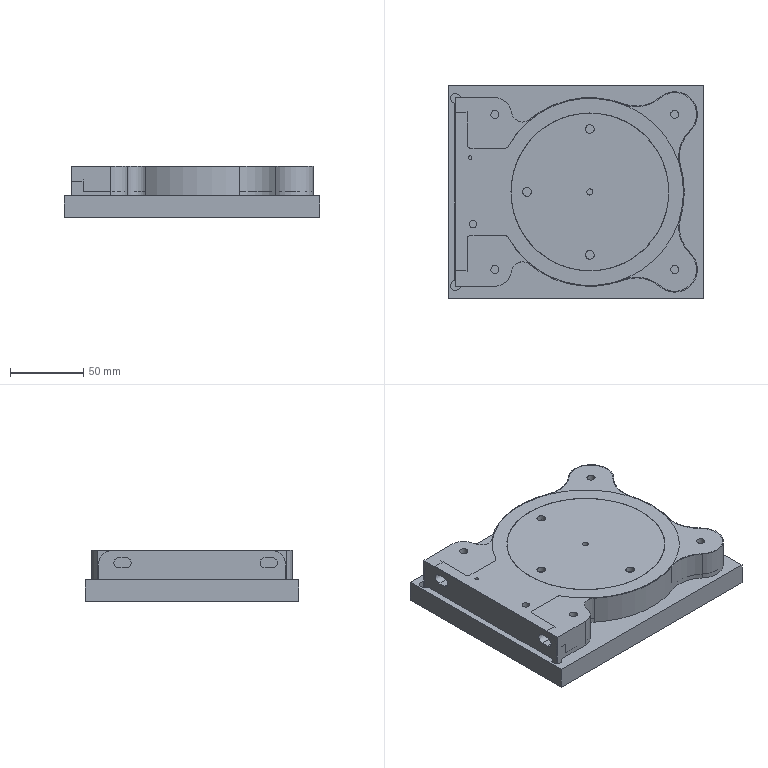NC program | NX | posted with a generic post | part box 175 x 146 x 35 mm
Lines 2956 to 4708 of 35144, first 1512 of 1711 lines:
(打点_COPY_COPY , TOOL : DJ6)
N5898 T12 M6
N5900 G54
N5902 G17 G0 G90 X67.5 Y-53. S3000 M3
N5904 G43 Z20. H12
N5906 G94 G81 G98 Z-1.2 F200. R3.
N5908 X-55.5
N5910 Y53.
N5912 X67.5
N5914 X9.5 Y0.
N5916 G80
N5918 G0 X9.5 Y0. Z20.
N5920 M5
(DRILLING_COPY_1 , TOOL : Z4.3)
N5922 T16 M6
N5924 G54
N5926 G17 G0 G90 X67.5 Y53. S3000 M3
N5928 G43 Z20. H16
N5930 G94 G83 G98 Z-15. F200. Q3. R3.
N5932 Y-53.
N5934 X9.5 Y0.
N5936 X-55.5 Y-53.
N5938 Y53.
N5940 G80
N5942 G0 X-55.5 Y53. Z20.
N5944 M5
(打点_COPY_COPY_COPY , TOOL : DJ6)
N5946 T12 M6
N5948 G54
N5950 G17 G0 G90 X67.5 Y-53. S3000 M3
N5952 G43 Z20. H12
N5954 G94 G81 G98 Z-2.5 F200. R3.
N5956 X-55.5
N5958 Y53.
N5960 X67.5
N5962 X9.5 Y0.
N5964 G80
N5966 G0 X9.5 Y0. Z20.
(倒角_COPY_1_COPY_2 , TOOL : DJ6)
N5968 X-73.2 Y0.249 S7500
N5970 Z-0.5
N5972 G1 Z-1. F1500.
N5974 G3 X-73.7 Y-0.251 R0.5
N5976 G1 Y-24.503
N5978 G2 X-73.993 Y-25.21 R1.
N5980 G1 X-74.288 Y-25.505
N5982 G3 X-74.288 Y-25.788 R0.2
N5984 X-74.005 Y-25.788 R0.2
N5986 G1 X-73.71 Y-25.493
N5988 G2 X-73.003 Y-25.2 R1.
N5990 G1 X-44.7
N5992 G2 X-43.799 Y-25.765 R1.
N5994 G3 X-43.799 Y25.765 R-59.2
N5996 G2 X-44.7 Y25.2 R1.
N5998 G1 X-72.5
N6000 G3 X-73.7 Y24. R1.2
N6002 G1 Y-0.251
N6004 G3 X-73.2 Y-0.751 R0.5
N6006 G1 Z-0.5
N6008 G0 Z20.
(倒角_COPY_1_COPY_2_COPY , TOOL : DJ6)
N6010 X-83.8 Y-0.5
N6012 Z-0.5
N6014 G1 Z-1.
N6016 G3 X-83.3 Y0. R0.5
N6018 G1 Y63.8
N6020 G2 X-82.3 Y64.8 R1.
N6022 G1 X-55.5
N6024 G2 X-43.785 Y54.413 R11.8
N6026 G3 X-32.023 Y49.748 R7.2
N6028 G2 X32.595 Y60.545 R64.8
N6030 G3 X57.119 Y64.911 R24.2
N6032 G2 X78.43 Y41.59 R15.8
N6034 G3 X71.876 Y17.558 R24.2
N6036 G2 X71.876 Y-17.558 R64.8
N6038 G3 X78.43 Y-41.59 R24.2
N6040 G2 X57.119 Y-64.911 R15.8
N6042 G3 X32.595 Y-60.545 R24.2
N6044 G2 X-32.023 Y-49.748 R64.8
N6046 G3 X-43.785 Y-54.413 R7.2
N6048 G2 X-55.5 Y-64.8 R11.8
N6050 G1 X-82.3
N6052 G2 X-83.3 Y-63.8 R1.
N6054 G1 Y0.
N6056 G3 X-83.8 Y0.5 R0.5
N6058 G1 Z-0.5
N6060 G0 Z20.
N6062 M5
(DRILLING_COPY_1_COPY , TOOL : M5)
N6064 T20 M6
N6066 G54
N6068 G17 G0 G90 X67.5 Y53. S300 M3
N6070 G43 Z20. H20
N6072 G84 G94 G98 Z-13. F72000. R3.
N6074 Y-53.
N6076 X9.5 Y0.
N6078 X-55.5 Y-53.
N6080 Y53.
N6082 G80
N6084 G0 X-55.5 Y53. Z20.
N6086 M5
(正面_COPY_COPY , TOOL : D10)
N6088 T02 M6
N6090 G54
N6092 G17 G0 G90 X95.5 Y-68.762 S8000 M3
N6094 G43 Z20. H2
N6096 Z0.1
N6098 G94 G1 X90.5 F1500.
N6100 X-90.5
N6102 Y-61.524
N6104 X90.5
N6106 Y-54.286
N6108 X-90.5
N6110 Y-47.048
N6112 X90.5
N6114 Y-39.81
N6116 X-90.5
N6118 Y-32.571
N6120 X90.5
N6122 Y-25.333
N6124 X-90.5
N6126 Y-18.095
N6128 X90.5
N6130 Y-10.857
N6132 X-90.5
N6134 Y-3.619
N6136 X90.5
N6138 Y3.619
N6140 X-90.5
N6142 Y10.857
N6144 X90.5
N6146 Y18.095
N6148 X-90.5
N6150 Y25.333
N6152 X90.5
N6154 Y32.571
N6156 X-90.5
N6158 Y39.81
N6160 X90.5
N6162 Y47.048
N6164 X-90.5
N6166 Y54.286
N6168 X90.5
N6170 Y61.524
N6172 X-90.5
N6174 Y68.762
N6176 X90.5
N6178 X95.5
N6180 G0 Z20.
(跟随部件_COPY_1_COPY_1 , TOOL : D10)
N6182 G1 X84.885 Y-72.393 F15000.
N6184 Z-26.5
N6186 Z-27. F1500.
N6188 G3 X78.03 Y-70.659 R5.
N6190 G2 X53.992 Y-68.5 R20.56
N6192 G3 X34.291 Y-64.992 R19.44
N6194 G2 X-35.073 Y-53.402 R69.56
N6196 G3 X-39.059 Y-54.983 R2.44
N6198 G2 X-55.5 Y-69.56 R16.56
N6200 G1 X-82.5
N6202 G2 X-88.06 Y-64. R5.56
N6204 G1 Y64.
N6206 G2 X-82.5 Y69.56 R5.56
N6208 G1 X-55.5
N6210 G2 X-39.059 Y54.983 R16.56
N6212 G3 X-35.073 Y53.402 R2.44
N6214 G2 X34.291 Y64.992 R69.56
N6216 G3 X53.992 Y68.5 R19.44
N6218 G2 X81.723 Y38.153 R20.56
N6220 G3 X76.458 Y18.848 R19.44
N6222 G2 X76.458 Y-18.848 R69.56
N6224 G3 X81.723 Y-38.153 R19.44
N6226 G2 X77.597 Y-70.91 R20.56
N6228 G3 X75.697 Y-77.721 R5.
N6230 G1 X84.854 Y-72.341
N6232 G3 X77.999 Y-70.607 R5.
N6234 G2 X54.031 Y-68.455 R20.5
N6236 G3 X34.27 Y-64.936 R19.5
N6238 G2 X-35.035 Y-53.356 R69.5
N6240 G3 X-39.119 Y-54.976 R2.5
N6242 G2 X-55.5 Y-69.5 R16.5
N6244 G1 X-82.5
N6246 G2 X-88. Y-64. R5.5
N6248 G1 Y64.
N6250 G2 X-82.5 Y69.5 R5.5
N6252 G1 X-55.5
N6254 G2 X-39.119 Y54.976 R16.5
N6256 G3 X-35.035 Y53.356 R2.5
N6258 G2 X34.27 Y64.936 R69.5
N6260 G3 X54.031 Y68.455 R19.5
N6262 G2 X81.681 Y38.197 R20.5
N6264 G3 X76.4 Y18.831 R19.5
N6266 G2 X76.4 Y-18.831 R69.5
N6268 G3 X81.681 Y-38.197 R19.5
N6270 G2 X77.999 Y-70.607 R20.5
N6272 X77.566 Y-70.858 R20.5
N6274 G3 X75.666 Y-77.669 R5.
N6276 G1 Z-26.5
N6278 Z20. F15000.
(反面_COPY , TOOL : D10)
N6280 G0 X-71.818 Y-98.5
N6282 Z3.4
N6284 G1 Y-93.5 F4000.
N6286 Y93.5
N6288 X-64.636
N6290 Y-93.5
N6292 X-57.455
N6294 Y93.5
N6296 X-50.273
N6298 Y-93.5
N6300 X-43.091
N6302 Y93.5
N6304 X-35.909
N6306 Y-93.5
N6308 X-28.727
N6310 Y93.5
N6312 X-21.545
N6314 Y-93.5
N6316 X-14.364
N6318 Y93.5
N6320 X-7.182
N6322 Y-93.5
N6324 X0.
N6326 Y93.5
N6328 X7.182
N6330 Y-93.5
N6332 X14.364
N6334 Y93.5
N6336 X21.545
N6338 Y-93.5
N6340 X28.727
N6342 Y93.5
N6344 X35.909
N6346 Y-93.5
N6348 X43.091
N6350 Y93.5
N6352 X50.273
N6354 Y-93.5
N6356 X57.455
N6358 Y93.5
N6360 X64.636
N6362 Y-93.5
N6364 X71.818
N6366 Y93.5
N6368 Y98.5
N6370 G0 Z8.
N6372 X-71.818 Y-98.5
N6374 Z1.8
N6376 G1 Y-93.5
N6378 Y93.5
N6380 X-64.636
N6382 Y-93.5
N6384 X-57.455
N6386 Y93.5
N6388 X-50.273
N6390 Y-93.5
N6392 X-43.091
N6394 Y93.5
N6396 X-35.909
N6398 Y-93.5
N6400 X-28.727
N6402 Y93.5
N6404 X-21.545
N6406 Y-93.5
N6408 X-14.364
N6410 Y93.5
N6412 X-7.182
N6414 Y-93.5
N6416 X0.
N6418 Y93.5
N6420 X7.182
N6422 Y-93.5
N6424 X14.364
N6426 Y93.5
N6428 X21.545
N6430 Y-93.5
N6432 X28.727
N6434 Y93.5
N6436 X35.909
N6438 Y-93.5
N6440 X43.091
N6442 Y93.5
N6444 X50.273
N6446 Y-93.5
N6448 X57.455
N6450 Y93.5
N6452 X64.636
N6454 Y-93.5
N6456 X71.818
N6458 Y93.5
N6460 Y98.5
N6462 G0 Z6.4
N6464 X-71.818 Y-98.5
N6466 Z0.2
N6468 G1 Y-93.5
N6470 Y93.5
N6472 X-64.636
N6474 Y-93.5
N6476 X-57.455
N6478 Y93.5
N6480 X-50.273
N6482 Y-93.5
N6484 X-43.091
N6486 Y93.5
N6488 X-35.909
N6490 Y-93.5
N6492 X-28.727
N6494 Y93.5
N6496 X-21.545
N6498 Y-93.5
N6500 X-14.364
N6502 Y93.5
N6504 X-7.182
N6506 Y-93.5
N6508 X0.
N6510 Y93.5
N6512 X7.182
N6514 Y-93.5
N6516 X14.364
N6518 Y93.5
N6520 X21.545
N6522 Y-93.5
N6524 X28.727
N6526 Y93.5
N6528 X35.909
N6530 Y-93.5
N6532 X43.091
N6534 Y93.5
N6536 X50.273
N6538 Y-93.5
N6540 X57.455
N6542 Y93.5
N6544 X64.636
N6546 Y-93.5
N6548 X71.818
N6550 Y93.5
N6552 Y98.5
N6554 G0 Z20.
(反面_COPY_COPY , TOOL : D10)
N6556 X-70.571 Y-97.5
N6558 Z0.1
N6560 G1 Y-92.5 F2000.
N6562 Y92.5
N6564 X-63.143
N6566 Y-92.5
N6568 X-55.714
N6570 Y92.5
N6572 X-48.286
N6574 Y-92.5
N6576 X-40.857
N6578 Y92.5
N6580 X-33.429
N6582 Y-92.5
N6584 X-26.
N6586 Y92.5
N6588 X-18.571
N6590 Y-92.5
N6592 X-11.143
N6594 Y92.5
N6596 X-3.714
N6598 Y-92.5
N6600 X3.714
N6602 Y92.5
N6604 X11.143
N6606 Y-92.5
N6608 X18.571
N6610 Y92.5
N6612 X26.
N6614 Y-92.5
N6616 X33.429
N6618 Y92.5
N6620 X40.857
N6622 Y-92.5
N6624 X48.286
N6626 Y92.5
N6628 X55.714
N6630 Y-92.5
N6632 X63.143
N6634 Y92.5
N6636 X70.571
N6638 Y-92.5
N6640 Y-97.5
N6642 G0 Z20.
N6644 M5
(打点_COPY_COPY_COPY_1 , TOOL : DJ8)
N6646 T12 M6
N6648 G54
N6650 G17 G0 G90 X53. Y-67.5 S3000 M3
N6652 G43 Z20. H12
N6654 G94 G81 G98 Z-1.2 F200. R3.
N6656 X-53.
N6658 X0. Y-9.5
N6660 X-53. Y55.5
N6662 X-22. Y70.5
N6664 X53. Y55.5
N6666 G80
N6668 G0 X53. Y55.5 Z20.
N6670 M5
(DRILLING_COPY_1_COPY_1 , TOOL : Z4.3)
N6672 T16 M6
N6674 G54
N6676 G17 G0 G90 X0. Y-9.5 S3000 M3
N6678 G43 Z20. H16
N6680 G94 G83 G98 Z-15. F200. Q3. R3.
N6682 G80
N6684 G0 X0. Y-9.5 Z20.
(DRILLING_COPY_1_COPY_1_COPY_1 , TOOL : Z4.3)
N6686 X53. Y-67.5
N6688 G83 Z-15. F200. Q3. R3.
N6690 X-53.
N6692 X53. Y55.5
N6694 X-53.
N6696 G80
N6698 G0 X-53. Y55.5 Z20.
N6700 M5
(打点_COPY_COPY_COPY_COPY , TOOL : DJ8)
N6702 T12 M6
N6704 G54
N6706 G17 G0 G90 X0. Y-9.5 S3000 M3
N6708 G43 Z20. H12
N6710 G94 G81 G98 Z-2.5 F200. R3.
N6712 X53. Y-67.5
N6714 X-53.
N6716 G80
N6718 G0 X-53. Y-67.5 Z20.
(打点_COPY_COPY_COPY_COPY_COPY , TOOL : DJ8)
N6720 X53. Y55.5
N6722 G81 Z-2.5 F200. R3.
N6724 X-53.
N6726 X-22. Y70.5
N6728 G80
N6730 G0 X-22. Y70.5 Z20.
(倒角_COPY_1_COPY_2_COPY_1 , TOOL : DJ8)
N6732 X-1. Y84.3 S7500
N6734 Z-0.5
N6736 G1 Z-1. F1500.
N6738 G3 X0. Y83.3 R1.
N6740 G1 X64.3
N6742 G2 X65.3 Y82.3 R1.
N6744 G1 Y55.5
N6746 G2 X54.473 Y43.289 R12.3
N6748 G3 X50.132 Y32.343 R6.7
N6750 G2 X61.012 Y-32.773 R65.3
N6752 G3 X65.288 Y-56.791 R23.7
N6754 G2 X41.229 Y-78.776 R16.3
N6756 G3 X17.693 Y-72.357 R23.7
N6758 G2 X-17.693 Y-72.357 R65.3
N6760 G3 X-41.229 Y-78.776 R23.7
N6762 G2 X-65.288 Y-56.791 R16.3
N6764 G3 X-61.012 Y-32.773 R23.7
N6766 G2 X-50.132 Y32.343 R65.3
N6768 G3 X-54.473 Y43.289 R6.7
N6770 G2 X-65.3 Y55.5 R12.3
N6772 G1 Y82.3
N6774 G2 X-64.3 Y83.3 R1.
N6776 G1 X0.
N6778 G3 X1. Y84.3 R1.
N6780 G1 Z-0.5
N6782 G0 Z20.
N6784 M5
(DRILLING_COPY_1_COPY_COPY , TOOL : M5)
N6786 T20 M6
N6788 G54
N6790 G17 G0 G90 X-53. Y-67.5 S300 M3
N6792 G43 Z20. H20
N6794 G84 G94 G98 Z-13.5 F72000. R3.
N6796 X53.
N6798 X0. Y-9.5
N6800 X53. Y55.5
N6802 X-53.
N6804 G80
N6806 G0 X-53. Y55.5 Z20.
N6808 M5
(跟随部件_COPY_3 , TOOL : D10)
N6810 T02 M6
N6812 G54
N6814 G17 G94 G1 G90 X-1.729 Y-10.159 F15000. S8000 M3
N6816 G43 Z20. H2
N6818 Z0.22
N6820 X-1.562 Y-10.595 Z0.204 F4000.
N6822 X-1.401 Y-11.033 Z0.187
N6824 X-0.95 Y-11.154 Z0.171
N6826 X-0.501 Y-11.281 Z0.155
N6828 X-0.179 Y-11.371 Z0.143
N6830 X0.179 Y-11.372 Z0.131
N6832 X0.501 Y-11.281 Z0.119
N6834 X0.95 Y-11.154 Z0.103
N6836 X1.401 Y-11.033 Z0.086
N6838 X1.562 Y-10.595 Z0.07
N6840 X1.729 Y-10.159 Z0.054
N6842 X1.848 Y-9.847 Z0.042
N6844 X1.854 Y-9.19 Z0.019
N6846 X1.635 Y-8.571 Z-0.004
N6848 X1.058 Y-7.881 Z-0.035
N6850 X0.348 Y-7.001 Z-0.075
N6852 X0. Y-6.556 Z-0.094
N6854 X-0.696 Y-7.447 Z-0.134
N6856 X-1.42 Y-8.315 Z-0.173
N6858 X-1.635 Y-8.571 Z-0.185
N6860 X-1.854 Y-9.19 Z-0.208
N6862 X-1.848 Y-9.847 Z-0.231
N6864 X-1.729 Y-10.159 Z-0.243
N6866 X-1.562 Y-10.595 Z-0.259
N6868 X-1.401 Y-11.033 Z-0.275
N6870 X-0.95 Y-11.154 Z-0.291
N6872 X-0.501 Y-11.281 Z-0.308
N6874 X-0.179 Y-11.371 Z-0.319
N6876 X0.179 Y-11.372 Z-0.332
N6878 X0.501 Y-11.281 Z-0.344
N6880 X0.95 Y-11.154 Z-0.36
N6882 X1.401 Y-11.033 Z-0.376
N6884 X1.562 Y-10.595 Z-0.392
N6886 X1.729 Y-10.159 Z-0.409
N6888 X1.848 Y-9.847 Z-0.42
N6890 X1.854 Y-9.19 Z-0.443
N6892 X1.635 Y-8.571 Z-0.466
N6894 X1.058 Y-7.881 Z-0.498
N6896 X0.348 Y-7.001 Z-0.537
N6898 X0. Y-6.556 Z-0.557
N6900 X-0.696 Y-7.447 Z-0.596
N6902 X-1.42 Y-8.315 Z-0.636
N6904 X-1.635 Y-8.571 Z-0.648
N6906 X-1.854 Y-9.19 Z-0.67
N6908 X-1.848 Y-9.847 Z-0.693
N6910 X-1.729 Y-10.159 Z-0.705
N6912 X-1.562 Y-10.595 Z-0.721
N6914 X-1.401 Y-11.033 Z-0.738
N6916 X-0.95 Y-11.154 Z-0.754
N6918 X-0.501 Y-11.281 Z-0.77
N6920 X-0.179 Y-11.371 Z-0.782
N6922 X0.179 Y-11.372 Z-0.794
N6924 X0.501 Y-11.281 Z-0.806
N6926 X0.95 Y-11.154 Z-0.822
N6928 X1.401 Y-11.033 Z-0.839
N6930 X1.562 Y-10.595 Z-0.855
N6932 X1.729 Y-10.159 Z-0.871
N6934 X1.848 Y-9.847 Z-0.883
N6936 X1.854 Y-9.19 Z-0.906
N6938 X1.635 Y-8.571 Z-0.929
N6940 X1.058 Y-7.881 Z-0.96
N6942 X0.703 Y-7.441 Z-0.98
N6944 G2 X0. Y-6.556 R70.15
N6946 X-1.42 Y-8.315 R70.15
N6948 G3 X-1.729 Y-10.159 R1.85
N6950 G2 X-1.401 Y-11.033 R87.15
N6952 X-0.501 Y-11.281 R87.15
N6954 G3 X0.501 Y-11.281 R1.85
N6956 G2 X1.401 Y-11.033 R87.15
N6958 X1.729 Y-10.159 R87.15
N6960 G3 X1.42 Y-8.315 R1.85
N6962 G2 X0.703 Y-7.441 R70.15
N6964 G1 X4.593 Y-4.299
N6966 G2 X0. Y2.153 R65.15
N6968 X-5.259 Y-5.111 R65.15
N6970 G3 X-6.4 Y-11.941 R6.85
N6972 G2 X-5.228 Y-15.221 R82.15
N6974 X-1.856 Y-16.094 R82.15
N6976 G3 X1.855 Y-16.094 R6.85
N6978 G2 X5.228 Y-15.221 R82.15
N6980 X6.4 Y-11.941 R82.15
N6982 G3 X5.259 Y-5.111 R6.85
N6984 G2 X4.593 Y-4.299 R65.15
N6986 G1 X10.427 Y0.413
N6988 G2 X0. Y20.262 R57.65
N6990 G1 X-1.351 Y25.076
N6992 G3 X-0.143 Y35.25 R55.15
N6994 G1 X0.143
N6996 G3 X1.351 Y25.076 R55.15
N6998 X-1.351 Y25.076 R5.
N7000 G1 X0. Y20.262
N7002 G2 X-11.017 Y-0.305 R57.65
N7004 G3 X-13.408 Y-14.614 R14.35
N7006 G2 X-11.113 Y-21.662 R74.65
N7008 X-3.888 Y-23.313 R74.65
N7010 G3 X3.887 Y-23.314 R14.35
N7012 G2 X11.113 Y-21.662 R74.65
N7014 X13.408 Y-14.614 R74.65
N7016 G3 X11.017 Y-0.305 R14.35
N7018 G2 X10.427 Y0.413 R57.65
N7020 G1 X16.262 Y5.126
N7022 G2 X5.256 Y40.25 R50.15
N7024 G1 X-5.256
N7026 G2 X-16.775 Y4.501 R50.15
N7028 G3 X-20.415 Y-17.287 R21.85
N7030 G2 X-17.246 Y-28.373 R67.15
N7032 X-5.92 Y-30.533 R67.15
N7034 G3 X5.919 Y-30.533 R21.85
N7036 G2 X17.246 Y-28.373 R67.15
N7038 X20.415 Y-17.287 R67.15
N7040 G3 X16.775 Y4.501 R21.85
N7042 G2 X16.262 Y5.126 R50.15
N7044 G1 X22.096 Y9.838
N7046 G2 X14.099 Y47.75 R42.65
N7048 G1 X-14.099
N7050 G2 X-22.533 Y9.307 R42.65
N7052 G3 X-27.423 Y-19.96 R29.35
N7054 G2 X-23.778 Y-35.522 R59.65
N7056 X-7.953 Y-37.752 R59.65
N7058 G3 X7.951 Y-37.752 R29.35
N7060 G2 X23.778 Y-35.522 R59.65
N7062 X27.423 Y-19.96 R59.65
N7064 G3 X22.533 Y9.307 R29.35
N7066 G2 X22.096 Y9.838 R42.65
N7068 G1 X27.931 Y14.551
N7070 G2 X25.458 Y55.25 R35.15
N7072 G1 X30.059 Y57.607
N7074 X25.458 Y55.25
N7076 X-25.458
N7078 X-30.059 Y57.607
N7080 X-25.458 Y55.25
N7082 G2 X-28.29 Y14.113 R35.15
N7084 G3 X-34.43 Y-22.633 R36.85
N7086 G2 X-31.055 Y-43.484 R52.15
N7088 X-9.985 Y-44.972 R52.15
N7090 G3 X9.984 Y-44.972 R36.85
N7092 G2 X31.055 Y-43.484 R52.15
N7094 X34.43 Y-22.633 R52.15
N7096 G3 X28.29 Y14.113 R36.85
N7098 G2 X27.931 Y14.551 R35.15
N7100 G1 X33.766 Y19.263
N7102 G2 X44.35 Y62.037 R27.65
N7104 G1 Y62.75
N7106 X-44.35
N7108 Y62.037
N7110 G2 X-34.048 Y18.919 R27.65
N7112 G3 X-41.438 Y-25.306 R44.35
N7114 G2 X-40.237 Y-53.533 R44.65
N7116 G1 X-43.947 Y-57.593
N7118 X-40.237 Y-53.533
N7120 G2 X-12.017 Y-52.191 R44.65
N7122 G3 X12.017 Y-52.191 R44.35
N7124 G2 X40.237 Y-53.533 R44.65
N7126 G1 X43.947 Y-57.593
N7128 X40.237 Y-53.533
N7130 G2 X41.438 Y-25.306 R44.65
N7132 G3 X34.048 Y18.919 R44.35
N7134 G2 X33.766 Y19.263 R27.65
N7136 G1 X39.6 Y23.976
N7138 G2 X51.85 Y56.493 R20.15
N7140 G1 Y70.25
N7142 X-51.85
N7144 Y56.493
N7146 G2 X-39.806 Y23.725 R20.15
N7148 G3 X-48.445 Y-27.98 R51.85
N7150 G2 X-55.149 Y-65.628 R37.15
N7152 G3 X-50.942 Y-69.472 R2.85
N7154 G2 X-14.049 Y-59.41 R37.15
N7156 G3 X14.049 Y-59.41 R51.85
N7158 G2 X50.942 Y-69.472 R37.15
N7160 G3 X55.149 Y-65.628 R2.85
N7162 G2 X48.445 Y-27.98 R37.15
N7164 G3 X39.806 Y23.725 R51.85
N7166 G2 X39.6 Y23.976 R20.15
N7168 G1 X45.435 Y28.688
N7170 G2 X53.761 Y49.196 R12.65
N7172 G3 X59.35 Y55.5 R6.35
N7174 G1 Y77.304
N7176 G2 X59.364 Y77.764 R7.75
N7178 X58.904 Y77.75 R7.75
N7180 G1 X-58.904
N7182 G2 X-59.364 Y77.764 R7.75
N7184 X-59.35 Y77.304 R7.75
N7186 G1 Y55.5
N7188 G3 X-53.761 Y49.196 R6.35
N7190 G2 X-45.564 Y28.531 R12.65
N7192 G3 X-55.453 Y-30.653 R59.35
N7194 G2 X-60.803 Y-60.7 R29.65
N7196 G3 X-45.526 Y-74.66 R10.35
N7198 G2 X-16.081 Y-66.63 R29.65
N7200 G3 X16.081 Y-66.63 R59.35
N7202 G2 X45.526 Y-74.66 R29.65
N7204 G3 X60.803 Y-60.7 R10.35
N7206 G2 X55.453 Y-30.653 R29.65
N7208 G3 X45.564 Y28.531 R59.35
N7210 G2 X45.435 Y28.688 R12.65
N7212 G3 X38.403 Y29.436 R5.
N7214 G1 Z-0.48
N7216 Z2. F15000.
N7218 X-1.729 Y-10.159
N7220 Z-0.76
N7222 X-1.562 Y-10.595 Z-0.776 F4000.
N7224 X-1.401 Y-11.033 Z-0.793
N7226 X-0.95 Y-11.154 Z-0.809
N7228 X-0.501 Y-11.281 Z-0.825
N7230 X-0.179 Y-11.371 Z-0.837
N7232 X0.179 Y-11.372 Z-0.849
N7234 X0.501 Y-11.281 Z-0.861
N7236 X0.95 Y-11.154 Z-0.877
N7238 X1.401 Y-11.033 Z-0.894
N7240 X1.562 Y-10.595 Z-0.91
N7242 X1.729 Y-10.159 Z-0.926
N7244 X1.848 Y-9.847 Z-0.938
N7246 X1.854 Y-9.19 Z-0.961
N7248 X1.635 Y-8.571 Z-0.984
N7250 X1.058 Y-7.881 Z-1.015
N7252 X0.348 Y-7.001 Z-1.055
N7254 X0. Y-6.556 Z-1.074
N7256 X-0.696 Y-7.447 Z-1.114
N7258 X-1.42 Y-8.315 Z-1.153
N7260 X-1.635 Y-8.571 Z-1.165
N7262 X-1.854 Y-9.19 Z-1.188
N7264 X-1.848 Y-9.847 Z-1.211
N7266 X-1.729 Y-10.159 Z-1.223
N7268 X-1.562 Y-10.595 Z-1.239
N7270 X-1.401 Y-11.033 Z-1.255
N7272 X-0.95 Y-11.154 Z-1.271
N7274 X-0.501 Y-11.281 Z-1.288
N7276 X-0.179 Y-11.371 Z-1.299
N7278 X0.179 Y-11.372 Z-1.312
N7280 X0.501 Y-11.281 Z-1.324
N7282 X0.95 Y-11.154 Z-1.34
N7284 X1.401 Y-11.033 Z-1.356
N7286 X1.562 Y-10.595 Z-1.372
N7288 X1.729 Y-10.159 Z-1.389
N7290 X1.848 Y-9.847 Z-1.4
N7292 X1.854 Y-9.19 Z-1.423
N7294 X1.635 Y-8.571 Z-1.446
N7296 X1.058 Y-7.881 Z-1.478
N7298 X0.348 Y-7.001 Z-1.517
N7300 X0. Y-6.556 Z-1.537
N7302 X-0.696 Y-7.447 Z-1.576
N7304 X-1.42 Y-8.315 Z-1.616
N7306 X-1.635 Y-8.571 Z-1.628
N7308 X-1.854 Y-9.19 Z-1.65
N7310 X-1.848 Y-9.847 Z-1.673
N7312 X-1.729 Y-10.159 Z-1.685
N7314 X-1.562 Y-10.595 Z-1.701
N7316 X-1.401 Y-11.033 Z-1.718
N7318 X-0.95 Y-11.154 Z-1.734
N7320 X-0.501 Y-11.281 Z-1.75
N7322 X-0.179 Y-11.371 Z-1.762
N7324 X0.179 Y-11.372 Z-1.774
N7326 X0.501 Y-11.281 Z-1.786
N7328 X0.95 Y-11.154 Z-1.802
N7330 X1.401 Y-11.033 Z-1.819
N7332 X1.562 Y-10.595 Z-1.835
N7334 X1.729 Y-10.159 Z-1.851
N7336 X1.848 Y-9.847 Z-1.863
N7338 X1.854 Y-9.19 Z-1.886
N7340 X1.635 Y-8.571 Z-1.909
N7342 X1.058 Y-7.881 Z-1.94
N7344 X0.703 Y-7.441 Z-1.96
N7346 G2 X0. Y-6.556 R70.15
N7348 X-1.42 Y-8.315 R70.15
N7350 G3 X-1.729 Y-10.159 R1.85
N7352 G2 X-1.401 Y-11.033 R87.15
N7354 X-0.501 Y-11.281 R87.15
N7356 G3 X0.501 Y-11.281 R1.85
N7358 G2 X1.401 Y-11.033 R87.15
N7360 X1.729 Y-10.159 R87.15
N7362 G3 X1.42 Y-8.315 R1.85
N7364 G2 X0.703 Y-7.441 R70.15
N7366 G1 X4.593 Y-4.299
N7368 G2 X0. Y2.153 R65.15
N7370 X-5.259 Y-5.111 R65.15
N7372 G3 X-6.4 Y-11.941 R6.85
N7374 G2 X-5.228 Y-15.221 R82.15
N7376 X-1.856 Y-16.094 R82.15
N7378 G3 X1.855 Y-16.094 R6.85
N7380 G2 X5.228 Y-15.221 R82.15
N7382 X6.4 Y-11.941 R82.15
N7384 G3 X5.259 Y-5.111 R6.85
N7386 G2 X4.593 Y-4.299 R65.15
N7388 G1 X10.427 Y0.413
N7390 G2 X0. Y20.262 R57.65
N7392 G1 X-1.351 Y25.076
N7394 G3 X-0.143 Y35.25 R55.15
N7396 G1 X0.143
N7398 G3 X1.351 Y25.076 R55.15
N7400 X-1.351 Y25.076 R5.
N7402 G1 X0. Y20.262
N7404 G2 X-11.017 Y-0.305 R57.65
N7406 G3 X-13.408 Y-14.614 R14.35
N7408 G2 X-11.113 Y-21.662 R74.65
N7410 X-3.888 Y-23.313 R74.65
N7412 G3 X3.887 Y-23.314 R14.35
N7414 G2 X11.113 Y-21.662 R74.65
N7416 X13.408 Y-14.614 R74.65
N7418 G3 X11.017 Y-0.305 R14.35
N7420 G2 X10.427 Y0.413 R57.65
N7422 G1 X16.262 Y5.126
N7424 G2 X5.256 Y40.25 R50.15
N7426 G1 X-5.256
N7428 G2 X-16.775 Y4.501 R50.15
N7430 G3 X-20.415 Y-17.287 R21.85
N7432 G2 X-17.246 Y-28.373 R67.15
N7434 X-5.92 Y-30.533 R67.15
N7436 G3 X5.919 Y-30.533 R21.85
N7438 G2 X17.246 Y-28.373 R67.15
N7440 X20.415 Y-17.287 R67.15
N7442 G3 X16.775 Y4.501 R21.85
N7444 G2 X16.262 Y5.126 R50.15
N7446 G1 X22.096 Y9.838
N7448 G2 X14.099 Y47.75 R42.65
N7450 G1 X-14.099
N7452 G2 X-22.533 Y9.307 R42.65
N7454 G3 X-27.423 Y-19.96 R29.35
N7456 G2 X-23.778 Y-35.522 R59.65
N7458 X-7.953 Y-37.752 R59.65
N7460 G3 X7.951 Y-37.752 R29.35
N7462 G2 X23.778 Y-35.522 R59.65
N7464 X27.423 Y-19.96 R59.65
N7466 G3 X22.533 Y9.307 R29.35
N7468 G2 X22.096 Y9.838 R42.65
N7470 G1 X27.931 Y14.551
N7472 G2 X25.458 Y55.25 R35.15
N7474 G1 X30.059 Y57.607
N7476 X25.458 Y55.25
N7478 X-25.458
N7480 X-30.059 Y57.607
N7482 X-25.458 Y55.25
N7484 G2 X-28.29 Y14.113 R35.15
N7486 G3 X-34.43 Y-22.633 R36.85
N7488 G2 X-31.055 Y-43.484 R52.15
N7490 X-9.985 Y-44.972 R52.15
N7492 G3 X9.984 Y-44.972 R36.85
N7494 G2 X31.055 Y-43.484 R52.15
N7496 X34.43 Y-22.633 R52.15
N7498 G3 X28.29 Y14.113 R36.85
N7500 G2 X27.931 Y14.551 R35.15
N7502 G1 X33.766 Y19.263
N7504 G2 X44.35 Y62.037 R27.65
N7506 G1 Y62.75
N7508 X-44.35
N7510 Y62.037
N7512 G2 X-34.048 Y18.919 R27.65
N7514 G3 X-41.438 Y-25.306 R44.35
N7516 G2 X-40.237 Y-53.533 R44.65
N7518 G1 X-43.947 Y-57.593
N7520 X-40.237 Y-53.533
N7522 G2 X-12.017 Y-52.191 R44.65
N7524 G3 X12.017 Y-52.191 R44.35
N7526 G2 X40.237 Y-53.533 R44.65
N7528 G1 X43.947 Y-57.593
N7530 X40.237 Y-53.533
N7532 G2 X41.438 Y-25.306 R44.65
N7534 G3 X34.048 Y18.919 R44.35
N7536 G2 X33.766 Y19.263 R27.65
N7538 G1 X39.6 Y23.976
N7540 G2 X51.85 Y56.493 R20.15
N7542 G1 Y70.25
N7544 X-51.85
N7546 Y56.493
N7548 G2 X-39.806 Y23.725 R20.15
N7550 G3 X-48.445 Y-27.98 R51.85
N7552 G2 X-55.149 Y-65.628 R37.15
N7554 G3 X-50.942 Y-69.472 R2.85
N7556 G2 X-14.049 Y-59.41 R37.15
N7558 G3 X14.049 Y-59.41 R51.85
N7560 G2 X50.942 Y-69.472 R37.15
N7562 G3 X55.149 Y-65.628 R2.85
N7564 G2 X48.445 Y-27.98 R37.15
N7566 G3 X39.806 Y23.725 R51.85
N7568 G2 X39.6 Y23.976 R20.15
N7570 G1 X45.435 Y28.688
N7572 G2 X53.761 Y49.196 R12.65
N7574 G3 X59.35 Y55.5 R6.35
N7576 G1 Y77.304
N7578 G2 X59.364 Y77.764 R7.75
N7580 X58.904 Y77.75 R7.75
N7582 G1 X-58.904
N7584 G2 X-59.364 Y77.764 R7.75
N7586 X-59.35 Y77.304 R7.75
N7588 G1 Y55.5
N7590 G3 X-53.761 Y49.196 R6.35
N7592 G2 X-45.564 Y28.531 R12.65
N7594 G3 X-55.453 Y-30.653 R59.35
N7596 G2 X-60.803 Y-60.7 R29.65
N7598 G3 X-45.526 Y-74.66 R10.35
N7600 G2 X-16.081 Y-66.63 R29.65
N7602 G3 X16.081 Y-66.63 R59.35
N7604 G2 X45.526 Y-74.66 R29.65
N7606 G3 X60.803 Y-60.7 R10.35
N7608 G2 X55.453 Y-30.653 R29.65
N7610 G3 X45.564 Y28.531 R59.35
N7612 G2 X45.435 Y28.688 R12.65
N7614 G3 X38.403 Y29.436 R5.
N7616 G1 Z-1.46
N7618 Z1.02 F15000.
N7620 X-1.729 Y-10.159
N7622 Z-1.74
N7624 X-1.562 Y-10.595 Z-1.756 F4000.
N7626 X-1.401 Y-11.033 Z-1.773
N7628 X-0.95 Y-11.154 Z-1.789
N7630 X-0.501 Y-11.281 Z-1.805
N7632 X-0.179 Y-11.371 Z-1.817
N7634 X0.179 Y-11.372 Z-1.829
N7636 X0.501 Y-11.281 Z-1.841
N7638 X0.95 Y-11.154 Z-1.857
N7640 X1.401 Y-11.033 Z-1.874
N7642 X1.562 Y-10.595 Z-1.89
N7644 X1.729 Y-10.159 Z-1.906
N7646 X1.848 Y-9.847 Z-1.918
N7648 X1.854 Y-9.19 Z-1.941
N7650 X1.635 Y-8.571 Z-1.964
N7652 X1.058 Y-7.881 Z-1.995
N7654 X0.348 Y-7.001 Z-2.035
N7656 X0. Y-6.556 Z-2.054
N7658 X-0.696 Y-7.447 Z-2.094
N7660 X-1.42 Y-8.315 Z-2.133
N7662 X-1.635 Y-8.571 Z-2.145
N7664 X-1.854 Y-9.19 Z-2.168
N7666 X-1.848 Y-9.847 Z-2.191
N7668 X-1.729 Y-10.159 Z-2.203
N7670 X-1.562 Y-10.595 Z-2.219
N7672 X-1.401 Y-11.033 Z-2.235
N7674 X-0.95 Y-11.154 Z-2.251
N7676 X-0.501 Y-11.281 Z-2.268
N7678 X-0.179 Y-11.371 Z-2.279
N7680 X0.179 Y-11.372 Z-2.292
N7682 X0.501 Y-11.281 Z-2.304
N7684 X0.95 Y-11.154 Z-2.32
N7686 X1.401 Y-11.033 Z-2.336
N7688 X1.562 Y-10.595 Z-2.352
N7690 X1.729 Y-10.159 Z-2.369
N7692 X1.848 Y-9.847 Z-2.38
N7694 X1.854 Y-9.19 Z-2.403
N7696 X1.635 Y-8.571 Z-2.426
N7698 X1.058 Y-7.881 Z-2.458
N7700 X0.348 Y-7.001 Z-2.497
N7702 X0. Y-6.556 Z-2.517
N7704 X-0.696 Y-7.447 Z-2.556
N7706 X-1.42 Y-8.315 Z-2.596
N7708 X-1.635 Y-8.571 Z-2.608
N7710 X-1.854 Y-9.19 Z-2.63
N7712 X-1.848 Y-9.847 Z-2.653
N7714 X-1.729 Y-10.159 Z-2.665
N7716 X-1.562 Y-10.595 Z-2.681
N7718 X-1.401 Y-11.033 Z-2.698
N7720 X-0.95 Y-11.154 Z-2.714
N7722 X-0.501 Y-11.281 Z-2.73
N7724 X-0.179 Y-11.371 Z-2.742
N7726 X0.179 Y-11.372 Z-2.754
N7728 X0.501 Y-11.281 Z-2.766
N7730 X0.95 Y-11.154 Z-2.782
N7732 X1.401 Y-11.033 Z-2.799
N7734 X1.562 Y-10.595 Z-2.815
N7736 X1.729 Y-10.159 Z-2.831
N7738 X1.848 Y-9.847 Z-2.843
N7740 X1.854 Y-9.19 Z-2.866
N7742 X1.635 Y-8.571 Z-2.889
N7744 X1.058 Y-7.881 Z-2.92
N7746 X0.703 Y-7.441 Z-2.94
N7748 G2 X0. Y-6.556 R70.15
N7750 X-1.42 Y-8.315 R70.15
N7752 G3 X-1.729 Y-10.159 R1.85
N7754 G2 X-1.401 Y-11.033 R87.15
N7756 X-0.501 Y-11.281 R87.15
N7758 G3 X0.501 Y-11.281 R1.85
N7760 G2 X1.401 Y-11.033 R87.15
N7762 X1.729 Y-10.159 R87.15
N7764 G3 X1.42 Y-8.315 R1.85
N7766 G2 X0.703 Y-7.441 R70.15
N7768 G1 X4.593 Y-4.299
N7770 G2 X0. Y2.153 R65.15
N7772 X-5.259 Y-5.111 R65.15
N7774 G3 X-6.4 Y-11.941 R6.85
N7776 G2 X-5.228 Y-15.221 R82.15
N7778 X-1.856 Y-16.094 R82.15
N7780 G3 X1.855 Y-16.094 R6.85
N7782 G2 X5.228 Y-15.221 R82.15
N7784 X6.4 Y-11.941 R82.15
N7786 G3 X5.259 Y-5.111 R6.85
N7788 G2 X4.593 Y-4.299 R65.15
N7790 G1 X10.427 Y0.413
N7792 G2 X0. Y20.262 R57.65
N7794 G1 X-1.351 Y25.076
N7796 G3 X-0.143 Y35.25 R55.15
N7798 G1 X0.143
N7800 G3 X1.351 Y25.076 R55.15
N7802 X-1.351 Y25.076 R5.
N7804 G1 X0. Y20.262
N7806 G2 X-11.017 Y-0.305 R57.65
N7808 G3 X-13.408 Y-14.614 R14.35
N7810 G2 X-11.113 Y-21.662 R74.65
N7812 X-3.888 Y-23.313 R74.65
N7814 G3 X3.887 Y-23.314 R14.35
N7816 G2 X11.113 Y-21.662 R74.65
N7818 X13.408 Y-14.614 R74.65
N7820 G3 X11.017 Y-0.305 R14.35
N7822 G2 X10.427 Y0.413 R57.65
N7824 G1 X16.262 Y5.126
N7826 G2 X5.256 Y40.25 R50.15
N7828 G1 X-5.256
N7830 G2 X-16.775 Y4.501 R50.15
N7832 G3 X-20.415 Y-17.287 R21.85
N7834 G2 X-17.246 Y-28.373 R67.15
N7836 X-5.92 Y-30.533 R67.15
N7838 G3 X5.919 Y-30.533 R21.85
N7840 G2 X17.246 Y-28.373 R67.15
N7842 X20.415 Y-17.287 R67.15
N7844 G3 X16.775 Y4.501 R21.85
N7846 G2 X16.262 Y5.126 R50.15
N7848 G1 X22.096 Y9.838
N7850 G2 X14.099 Y47.75 R42.65
N7852 G1 X-14.099
N7854 G2 X-22.533 Y9.307 R42.65
N7856 G3 X-27.423 Y-19.96 R29.35
N7858 G2 X-23.778 Y-35.522 R59.65
N7860 X-7.953 Y-37.752 R59.65
N7862 G3 X7.951 Y-37.752 R29.35
N7864 G2 X23.778 Y-35.522 R59.65
N7866 X27.423 Y-19.96 R59.65
N7868 G3 X22.533 Y9.307 R29.35
N7870 G2 X22.096 Y9.838 R42.65
N7872 G1 X27.931 Y14.551
N7874 G2 X25.458 Y55.25 R35.15
N7876 G1 X30.059 Y57.607
N7878 X25.458 Y55.25
N7880 X-25.458
N7882 X-30.059 Y57.607
N7884 X-25.458 Y55.25
N7886 G2 X-28.29 Y14.113 R35.15
N7888 G3 X-34.43 Y-22.633 R36.85
N7890 G2 X-31.055 Y-43.484 R52.15
N7892 X-9.985 Y-44.972 R52.15
N7894 G3 X9.984 Y-44.972 R36.85
N7896 G2 X31.055 Y-43.484 R52.15
N7898 X34.43 Y-22.633 R52.15
N7900 G3 X28.29 Y14.113 R36.85
N7902 G2 X27.931 Y14.551 R35.15
N7904 G1 X33.766 Y19.263
N7906 G2 X44.35 Y62.037 R27.65
N7908 G1 Y62.75
N7910 X-44.35
N7912 Y62.037
N7914 G2 X-34.048 Y18.919 R27.65
N7916 G3 X-41.438 Y-25.306 R44.35
N7918 G2 X-40.237 Y-53.533 R44.65
N7920 G1 X-43.947 Y-57.593
N7922 X-40.237 Y-53.533
N7924 G2 X-12.017 Y-52.191 R44.65
N7926 G3 X12.017 Y-52.191 R44.35
N7928 G2 X40.237 Y-53.533 R44.65
N7930 G1 X43.947 Y-57.593
N7932 X40.237 Y-53.533
N7934 G2 X41.438 Y-25.306 R44.65
N7936 G3 X34.048 Y18.919 R44.35
N7938 G2 X33.766 Y19.263 R27.65
N7940 G1 X39.6 Y23.976
N7942 G2 X51.85 Y56.493 R20.15
N7944 G1 Y70.25
N7946 X-51.85
N7948 Y56.493
N7950 G2 X-39.806 Y23.725 R20.15
N7952 G3 X-48.445 Y-27.98 R51.85
N7954 G2 X-55.149 Y-65.628 R37.15
N7956 G3 X-50.942 Y-69.472 R2.85
N7958 G2 X-14.049 Y-59.41 R37.15
N7960 G3 X14.049 Y-59.41 R51.85
N7962 G2 X50.942 Y-69.472 R37.15
N7964 G3 X55.149 Y-65.628 R2.85
N7966 G2 X48.445 Y-27.98 R37.15
N7968 G3 X39.806 Y23.725 R51.85
N7970 G2 X39.6 Y23.976 R20.15
N7972 G1 X45.435 Y28.688
N7974 G2 X53.761 Y49.196 R12.65
N7976 G3 X59.35 Y55.5 R6.35
N7978 G1 Y77.304
N7980 G2 X59.364 Y77.764 R7.75
N7982 X58.904 Y77.75 R7.75
N7984 G1 X-58.904
N7986 G2 X-59.364 Y77.764 R7.75
N7988 X-59.35 Y77.304 R7.75
N7990 G1 Y55.5
N7992 G3 X-53.761 Y49.196 R6.35
N7994 G2 X-45.564 Y28.531 R12.65
N7996 G3 X-55.453 Y-30.653 R59.35
N7998 G2 X-60.803 Y-60.7 R29.65
N8000 G3 X-45.526 Y-74.66 R10.35
N8002 G2 X-16.081 Y-66.63 R29.65
N8004 G3 X16.081 Y-66.63 R59.35
N8006 G2 X45.526 Y-74.66 R29.65
N8008 G3 X60.803 Y-60.7 R10.35
N8010 G2 X55.453 Y-30.653 R29.65
N8012 G3 X45.564 Y28.531 R59.35
N8014 G2 X45.435 Y28.688 R12.65
N8016 G3 X38.403 Y29.436 R5.
N8018 G1 Z-2.44
N8020 Z0.04 F15000.
N8022 X-1.729 Y-10.159
N8024 Z-2.72
N8026 X-1.562 Y-10.595 Z-2.736 F4000.
N8028 X-1.401 Y-11.033 Z-2.753
N8030 X-0.95 Y-11.154 Z-2.769
N8032 X-0.501 Y-11.281 Z-2.785
N8034 X-0.179 Y-11.371 Z-2.797
N8036 X0.179 Y-11.372 Z-2.809
N8038 X0.501 Y-11.281 Z-2.821
N8040 X0.95 Y-11.154 Z-2.837
N8042 X1.401 Y-11.033 Z-2.854
N8044 X1.562 Y-10.595 Z-2.87
N8046 X1.729 Y-10.159 Z-2.886
N8048 X1.848 Y-9.847 Z-2.898
N8050 X1.854 Y-9.19 Z-2.921
N8052 X1.635 Y-8.571 Z-2.944
N8054 X1.058 Y-7.881 Z-2.975
N8056 X0.348 Y-7.001 Z-3.015
N8058 X0. Y-6.556 Z-3.034
N8060 X-0.696 Y-7.447 Z-3.074
N8062 X-1.42 Y-8.315 Z-3.113
N8064 X-1.635 Y-8.571 Z-3.125
N8066 X-1.854 Y-9.19 Z-3.148
N8068 X-1.848 Y-9.847 Z-3.171
N8070 X-1.729 Y-10.159 Z-3.183
N8072 X-1.562 Y-10.595 Z-3.199
N8074 X-1.401 Y-11.033 Z-3.215
N8076 X-0.95 Y-11.154 Z-3.231
N8078 X-0.501 Y-11.281 Z-3.248
N8080 X-0.179 Y-11.371 Z-3.259
N8082 X0.179 Y-11.372 Z-3.272
N8084 X0.501 Y-11.281 Z-3.284
N8086 X0.95 Y-11.154 Z-3.3
N8088 X1.401 Y-11.033 Z-3.316
N8090 X1.562 Y-10.595 Z-3.332
N8092 X1.729 Y-10.159 Z-3.349
N8094 X1.848 Y-9.847 Z-3.36
N8096 X1.854 Y-9.19 Z-3.383
N8098 X1.635 Y-8.571 Z-3.406
N8100 X1.058 Y-7.881 Z-3.438
N8102 X0.348 Y-7.001 Z-3.477
N8104 X0. Y-6.556 Z-3.497
N8106 X-0.696 Y-7.447 Z-3.536
N8108 X-1.42 Y-8.315 Z-3.576
N8110 X-1.635 Y-8.571 Z-3.588
N8112 X-1.854 Y-9.19 Z-3.61
N8114 X-1.848 Y-9.847 Z-3.633
N8116 X-1.729 Y-10.159 Z-3.645
N8118 X-1.562 Y-10.595 Z-3.661
N8120 X-1.401 Y-11.033 Z-3.678
N8122 X-0.95 Y-11.154 Z-3.694
N8124 X-0.501 Y-11.281 Z-3.71
N8126 X-0.179 Y-11.371 Z-3.722
N8128 X0.179 Y-11.372 Z-3.734
N8130 X0.501 Y-11.281 Z-3.746
N8132 X0.95 Y-11.154 Z-3.762
N8134 X1.401 Y-11.033 Z-3.779
N8136 X1.562 Y-10.595 Z-3.795
N8138 X1.729 Y-10.159 Z-3.811
N8140 X1.848 Y-9.847 Z-3.823
N8142 X1.854 Y-9.19 Z-3.846
N8144 X1.635 Y-8.571 Z-3.869
N8146 X1.058 Y-7.881 Z-3.9
N8148 X0.703 Y-7.441 Z-3.92
N8150 G2 X0. Y-6.556 R70.15
N8152 X-1.42 Y-8.315 R70.15
N8154 G3 X-1.729 Y-10.159 R1.85
N8156 G2 X-1.401 Y-11.033 R87.15
N8158 X-0.501 Y-11.281 R87.15
N8160 G3 X0.501 Y-11.281 R1.85
N8162 G2 X1.401 Y-11.033 R87.15
N8164 X1.729 Y-10.159 R87.15
N8166 G3 X1.42 Y-8.315 R1.85
N8168 G2 X0.703 Y-7.441 R70.15
N8170 G1 X4.593 Y-4.299
N8172 G2 X0. Y2.153 R65.15
N8174 X-5.259 Y-5.111 R65.15
N8176 G3 X-6.4 Y-11.941 R6.85
N8178 G2 X-5.228 Y-15.221 R82.15
N8180 X-1.856 Y-16.094 R82.15
N8182 G3 X1.855 Y-16.094 R6.85
N8184 G2 X5.228 Y-15.221 R82.15
N8186 X6.4 Y-11.941 R82.15
N8188 G3 X5.259 Y-5.111 R6.85
N8190 G2 X4.593 Y-4.299 R65.15
N8192 G1 X10.427 Y0.413
N8194 G2 X0. Y20.262 R57.65
N8196 G1 X-1.351 Y25.076
N8198 G3 X-0.143 Y35.25 R55.15
N8200 G1 X0.143
N8202 G3 X1.351 Y25.076 R55.15
N8204 X-1.351 Y25.076 R5.
N8206 G1 X0. Y20.262
N8208 G2 X-11.017 Y-0.305 R57.65
N8210 G3 X-13.408 Y-14.614 R14.35
N8212 G2 X-11.113 Y-21.662 R74.65
N8214 X-3.888 Y-23.313 R74.65
N8216 G3 X3.887 Y-23.314 R14.35
N8218 G2 X11.113 Y-21.662 R74.65
N8220 X13.408 Y-14.614 R74.65
N8222 G3 X11.017 Y-0.305 R14.35
N8224 G2 X10.427 Y0.413 R57.65
N8226 G1 X16.262 Y5.126
N8228 G2 X5.256 Y40.25 R50.15
N8230 G1 X-5.256
N8232 G2 X-16.775 Y4.501 R50.15
N8234 G3 X-20.415 Y-17.287 R21.85
N8236 G2 X-17.246 Y-28.373 R67.15
N8238 X-5.92 Y-30.533 R67.15
N8240 G3 X5.919 Y-30.533 R21.85
N8242 G2 X17.246 Y-28.373 R67.15
N8244 X20.415 Y-17.287 R67.15
N8246 G3 X16.775 Y4.501 R21.85
N8248 G2 X16.262 Y5.126 R50.15
N8250 G1 X22.096 Y9.838
N8252 G2 X14.099 Y47.75 R42.65
N8254 G1 X-14.099
N8256 G2 X-22.533 Y9.307 R42.65
N8258 G3 X-27.423 Y-19.96 R29.35
N8260 G2 X-23.778 Y-35.522 R59.65
N8262 X-7.953 Y-37.752 R59.65
N8264 G3 X7.951 Y-37.752 R29.35
N8266 G2 X23.778 Y-35.522 R59.65
N8268 X27.423 Y-19.96 R59.65
N8270 G3 X22.533 Y9.307 R29.35
N8272 G2 X22.096 Y9.838 R42.65
N8274 G1 X27.931 Y14.551
N8276 G2 X25.458 Y55.25 R35.15
N8278 G1 X30.059 Y57.607
N8280 X25.458 Y55.25
N8282 X-25.458
N8284 X-30.059 Y57.607
N8286 X-25.458 Y55.25
N8288 G2 X-28.29 Y14.113 R35.15
N8290 G3 X-34.43 Y-22.633 R36.85
N8292 G2 X-31.055 Y-43.484 R52.15
N8294 X-9.985 Y-44.972 R52.15
N8296 G3 X9.984 Y-44.972 R36.85
N8298 G2 X31.055 Y-43.484 R52.15
N8300 X34.43 Y-22.633 R52.15
N8302 G3 X28.29 Y14.113 R36.85
N8304 G2 X27.931 Y14.551 R35.15
N8306 G1 X33.766 Y19.263
N8308 G2 X44.35 Y62.037 R27.65
N8310 G1 Y62.75
N8312 X-44.35
N8314 Y62.037
N8316 G2 X-34.048 Y18.919 R27.65
N8318 G3 X-41.438 Y-25.306 R44.35
N8320 G2 X-40.237 Y-53.533 R44.65
N8322 G1 X-43.947 Y-57.593
N8324 X-40.237 Y-53.533
N8326 G2 X-12.017 Y-52.191 R44.65
N8328 G3 X12.017 Y-52.191 R44.35
N8330 G2 X40.237 Y-53.533 R44.65
N8332 G1 X43.947 Y-57.593
N8334 X40.237 Y-53.533
N8336 G2 X41.438 Y-25.306 R44.65
N8338 G3 X34.048 Y18.919 R44.35
N8340 G2 X33.766 Y19.263 R27.65
N8342 G1 X39.6 Y23.976
N8344 G2 X51.85 Y56.493 R20.15
N8346 G1 Y70.25
N8348 X-51.85
N8350 Y56.493
N8352 G2 X-39.806 Y23.725 R20.15
N8354 G3 X-48.445 Y-27.98 R51.85
N8356 G2 X-55.149 Y-65.628 R37.15
N8358 G3 X-50.942 Y-69.472 R2.85
N8360 G2 X-14.049 Y-59.41 R37.15
N8362 G3 X14.049 Y-59.41 R51.85
N8364 G2 X50.942 Y-69.472 R37.15
N8366 G3 X55.149 Y-65.628 R2.85
N8368 G2 X48.445 Y-27.98 R37.15
N8370 G3 X39.806 Y23.725 R51.85
N8372 G2 X39.6 Y23.976 R20.15
N8374 G1 X45.435 Y28.688
N8376 G2 X53.761 Y49.196 R12.65
N8378 G3 X59.35 Y55.5 R6.35
N8380 G1 Y77.304
N8382 G2 X59.364 Y77.764 R7.75
N8384 X58.904 Y77.75 R7.75
N8386 G1 X-58.904
N8388 G2 X-59.364 Y77.764 R7.75
N8390 X-59.35 Y77.304 R7.75
N8392 G1 Y55.5
N8394 G3 X-53.761 Y49.196 R6.35
N8396 G2 X-45.564 Y28.531 R12.65
N8398 G3 X-55.453 Y-30.653 R59.35
N8400 G2 X-60.803 Y-60.7 R29.65
N8402 G3 X-45.526 Y-74.66 R10.35
N8404 G2 X-16.081 Y-66.63 R29.65
N8406 G3 X16.081 Y-66.63 R59.35
N8408 G2 X45.526 Y-74.66 R29.65
N8410 G3 X60.803 Y-60.7 R10.35
N8412 G2 X55.453 Y-30.653 R29.65
N8414 G3 X45.564 Y28.531 R59.35
N8416 G2 X45.435 Y28.688 R12.65
N8418 G3 X38.403 Y29.436 R5.
N8420 G1 Z-3.42
N8422 Z-0.94 F15000.
N8424 X-1.729 Y-10.159
N8426 Z-3.7
N8428 X-1.562 Y-10.595 Z-3.716 F4000.
N8430 X-1.401 Y-11.033 Z-3.733
N8432 X-0.95 Y-11.154 Z-3.749
N8434 X-0.501 Y-11.281 Z-3.765
N8436 X-0.179 Y-11.371 Z-3.777
N8438 X0.179 Y-11.372 Z-3.789
N8440 X0.501 Y-11.281 Z-3.801
N8442 X0.95 Y-11.154 Z-3.817
N8444 X1.401 Y-11.033 Z-3.834
N8446 X1.562 Y-10.595 Z-3.85
N8448 X1.729 Y-10.159 Z-3.866
N8450 X1.848 Y-9.847 Z-3.878
N8452 X1.854 Y-9.19 Z-3.901
N8454 X1.635 Y-8.571 Z-3.924
N8456 X1.058 Y-7.881 Z-3.955
N8458 X0.348 Y-7.001 Z-3.995
N8460 X0. Y-6.556 Z-4.014
N8462 X-0.696 Y-7.447 Z-4.054
N8464 X-1.42 Y-8.315 Z-4.093
N8466 X-1.635 Y-8.571 Z-4.105
N8468 X-1.854 Y-9.19 Z-4.128
N8470 X-1.848 Y-9.847 Z-4.151
N8472 X-1.729 Y-10.159 Z-4.163
N8474 X-1.562 Y-10.595 Z-4.179
N8476 X-1.401 Y-11.033 Z-4.195
N8478 X-0.95 Y-11.154 Z-4.211
N8480 X-0.501 Y-11.281 Z-4.228
N8482 X-0.179 Y-11.371 Z-4.239
N8484 X0.179 Y-11.372 Z-4.252
N8486 X0.501 Y-11.281 Z-4.264
N8488 X0.95 Y-11.154 Z-4.28
N8490 X1.401 Y-11.033 Z-4.296
N8492 X1.562 Y-10.595 Z-4.312
N8494 X1.729 Y-10.159 Z-4.329
N8496 X1.848 Y-9.847 Z-4.34
N8498 X1.854 Y-9.19 Z-4.363
N8500 X1.635 Y-8.571 Z-4.386
N8502 X1.058 Y-7.881 Z-4.418
N8504 X0.348 Y-7.001 Z-4.457
N8506 X0. Y-6.556 Z-4.477
N8508 X-0.696 Y-7.447 Z-4.516
N8510 X-1.42 Y-8.315 Z-4.556
N8512 X-1.635 Y-8.571 Z-4.568
N8514 X-1.854 Y-9.19 Z-4.59
N8516 X-1.848 Y-9.847 Z-4.613
N8518 X-1.729 Y-10.159 Z-4.625
N8520 X-1.562 Y-10.595 Z-4.641
N8522 X-1.401 Y-11.033 Z-4.658
N8524 X-0.95 Y-11.154 Z-4.674
N8526 X-0.501 Y-11.281 Z-4.69
N8528 X-0.179 Y-11.371 Z-4.702
N8530 X0.179 Y-11.372 Z-4.714
N8532 X0.501 Y-11.281 Z-4.726
N8534 X0.95 Y-11.154 Z-4.742
N8536 X1.401 Y-11.033 Z-4.759
N8538 X1.562 Y-10.595 Z-4.775
N8540 X1.729 Y-10.159 Z-4.791
N8542 X1.848 Y-9.847 Z-4.803
N8544 X1.854 Y-9.19 Z-4.826
N8546 X1.635 Y-8.571 Z-4.849
N8548 X1.058 Y-7.881 Z-4.88
N8550 X0.703 Y-7.441 Z-4.9
N8552 G2 X0. Y-6.556 R70.15
N8554 X-1.42 Y-8.315 R70.15
N8556 G3 X-1.729 Y-10.159 R1.85
N8558 G2 X-1.401 Y-11.033 R87.15
N8560 X-0.501 Y-11.281 R87.15
N8562 G3 X0.501 Y-11.281 R1.85
N8564 G2 X1.401 Y-11.033 R87.15
N8566 X1.729 Y-10.159 R87.15
N8568 G3 X1.42 Y-8.315 R1.85
N8570 G2 X0.703 Y-7.441 R70.15
N8572 G1 X4.593 Y-4.299
N8574 G2 X0. Y2.153 R65.15
N8576 X-5.259 Y-5.111 R65.15
N8578 G3 X-6.4 Y-11.941 R6.85
N8580 G2 X-5.228 Y-15.221 R82.15
N8582 X-1.856 Y-16.094 R82.15
N8584 G3 X1.855 Y-16.094 R6.85
N8586 G2 X5.228 Y-15.221 R82.15
N8588 X6.4 Y-11.941 R82.15
N8590 G3 X5.259 Y-5.111 R6.85
N8592 G2 X4.593 Y-4.299 R65.15
N8594 G1 X10.427 Y0.413
N8596 G2 X0. Y20.262 R57.65
N8598 G1 X-1.351 Y25.076
N8600 G3 X-0.143 Y35.25 R55.15
N8602 G1 X0.143
N8604 G3 X1.351 Y25.076 R55.15
N8606 X-1.351 Y25.076 R5.
N8608 G1 X0. Y20.262
N8610 G2 X-11.017 Y-0.305 R57.65
N8612 G3 X-13.408 Y-14.614 R14.35
N8614 G2 X-11.113 Y-21.662 R74.65
N8616 X-3.888 Y-23.313 R74.65
N8618 G3 X3.887 Y-23.314 R14.35
N8620 G2 X11.113 Y-21.662 R74.65
N8622 X13.408 Y-14.614 R74.65
N8624 G3 X11.017 Y-0.305 R14.35
N8626 G2 X10.427 Y0.413 R57.65
N8628 G1 X16.262 Y5.126
N8630 G2 X5.256 Y40.25 R50.15
N8632 G1 X-5.256
N8634 G2 X-16.775 Y4.501 R50.15
N8636 G3 X-20.415 Y-17.287 R21.85
N8638 G2 X-17.246 Y-28.373 R67.15
N8640 X-5.92 Y-30.533 R67.15
N8642 G3 X5.919 Y-30.533 R21.85
N8644 G2 X17.246 Y-28.373 R67.15
N8646 X20.415 Y-17.287 R67.15
N8648 G3 X16.775 Y4.501 R21.85
N8650 G2 X16.262 Y5.126 R50.15
N8652 G1 X22.096 Y9.838
N8654 G2 X14.099 Y47.75 R42.65
N8656 G1 X-14.099
N8658 G2 X-22.533 Y9.307 R42.65
N8660 G3 X-27.423 Y-19.96 R29.35
N8662 G2 X-23.778 Y-35.522 R59.65
N8664 X-7.953 Y-37.752 R59.65
N8666 G3 X7.951 Y-37.752 R29.35
N8668 G2 X23.778 Y-35.522 R59.65
N8670 X27.423 Y-19.96 R59.65
N8672 G3 X22.533 Y9.307 R29.35
N8674 G2 X22.096 Y9.838 R42.65
N8676 G1 X27.931 Y14.551
N8678 G2 X25.458 Y55.25 R35.15
N8680 G1 X30.059 Y57.607
N8682 X25.458 Y55.25
N8684 X-25.458
N8686 X-30.059 Y57.607
N8688 X-25.458 Y55.25
N8690 G2 X-28.29 Y14.113 R35.15
N8692 G3 X-34.43 Y-22.633 R36.85
N8694 G2 X-31.055 Y-43.484 R52.15
N8696 X-9.985 Y-44.972 R52.15
N8698 G3 X9.984 Y-44.972 R36.85
N8700 G2 X31.055 Y-43.484 R52.15
N8702 X34.43 Y-22.633 R52.15
N8704 G3 X28.29 Y14.113 R36.85
N8706 G2 X27.931 Y14.551 R35.15
N8708 G1 X33.766 Y19.263
N8710 G2 X44.35 Y62.037 R27.65
N8712 G1 Y62.75
N8714 X-44.35
N8716 Y62.037
N8718 G2 X-34.048 Y18.919 R27.65
N8720 G3 X-41.438 Y-25.306 R44.35
N8722 G2 X-40.237 Y-53.533 R44.65
N8724 G1 X-43.947 Y-57.593
N8726 X-40.237 Y-53.533
N8728 G2 X-12.017 Y-52.191 R44.65
N8730 G3 X12.017 Y-52.191 R44.35
N8732 G2 X40.237 Y-53.533 R44.65
N8734 G1 X43.947 Y-57.593
N8736 X40.237 Y-53.533
N8738 G2 X41.438 Y-25.306 R44.65
N8740 G3 X34.048 Y18.919 R44.35
N8742 G2 X33.766 Y19.263 R27.65
N8744 G1 X39.6 Y23.976
N8746 G2 X51.85 Y56.493 R20.15
N8748 G1 Y70.25
N8750 X-51.85
N8752 Y56.493
N8754 G2 X-39.806 Y23.725 R20.15
N8756 G3 X-48.445 Y-27.98 R51.85
N8758 G2 X-55.149 Y-65.628 R37.15
N8760 G3 X-50.942 Y-69.472 R2.85
N8762 G2 X-14.049 Y-59.41 R37.15
N8764 G3 X14.049 Y-59.41 R51.85
N8766 G2 X50.942 Y-69.472 R37.15
N8768 G3 X55.149 Y-65.628 R2.85
N8770 G2 X48.445 Y-27.98 R37.15
N8772 G3 X39.806 Y23.725 R51.85
N8774 G2 X39.6 Y23.976 R20.15
N8776 G1 X45.435 Y28.688
N8778 G2 X53.761 Y49.196 R12.65
N8780 G3 X59.35 Y55.5 R6.35
N8782 G1 Y77.304
N8784 G2 X59.364 Y77.764 R7.75
N8786 X58.904 Y77.75 R7.75
N8788 G1 X-58.904
N8790 G2 X-59.364 Y77.764 R7.75
N8792 X-59.35 Y77.304 R7.75
N8794 G1 Y55.5
N8796 G3 X-53.761 Y49.196 R6.35
N8798 G2 X-45.564 Y28.531 R12.65
N8800 G3 X-55.453 Y-30.653 R59.35
N8802 G2 X-60.803 Y-60.7 R29.65
N8804 G3 X-45.526 Y-74.66 R10.35
N8806 G2 X-16.081 Y-66.63 R29.65
N8808 G3 X16.081 Y-66.63 R59.35
N8810 G2 X45.526 Y-74.66 R29.65
N8812 G3 X60.803 Y-60.7 R10.35
N8814 G2 X55.453 Y-30.653 R29.65
N8816 G3 X45.564 Y28.531 R59.35
N8818 G2 X45.435 Y28.688 R12.65
N8820 G3 X38.403 Y29.436 R5.
N8822 G1 Z-4.4
N8824 Z20. F15000.
(底壁_COPY_COPY_1 , TOOL : D10)
N8826 G0 X0.706 Y-11.584 S8500
N8828 Z-4.5
N8830 G1 Z-5. F1500.
N8832 G3 X1.626 Y-4.573 R5.
N8834 G2 X0. Y-2.365 R67.65
N8836 X-3.334 Y-6.706 R67.65
N8838 G3 X-4.064 Y-11.05 R4.35
N8840 G2 X-3.306 Y-13.118 R84.65
N8842 X-1.179 Y-13.687 R84.65
N8844 G3 X1.179 Y-13.687 R4.35
N8846 G2 X3.306 Y-13.118 R84.65
N8848 X4.064 Y-11.05 R84.65
N8850 G3 X3.34 Y-6.713 R4.35
N8852 G2 X1.626 Y-4.573 R67.65
N8854 G1 X5.988 Y-1.222
N8856 G2 X0. Y8.225 R62.15
N8858 X-7.557 Y-3.182 R62.15
N8860 G3 X-9.203 Y-13.011 R9.85
N8862 G2 X-7.559 Y-17.772 R79.15
N8864 X-2.669 Y-18.982 R79.15
N8866 G3 X2.669 Y-18.982 R9.85
N8868 G2 X7.559 Y-17.772 R79.15
N8870 X9.203 Y-13.011 R79.15
N8872 G3 X7.562 Y-3.188 R9.85
N8874 G2 X5.988 Y-1.222 R62.15
N8876 G1 X10.349 Y2.128
N8878 G2 X0. Y24.234 R56.65
N8880 X-11.78 Y0.341 R56.65
N8882 G3 X-14.342 Y-14.971 R15.35